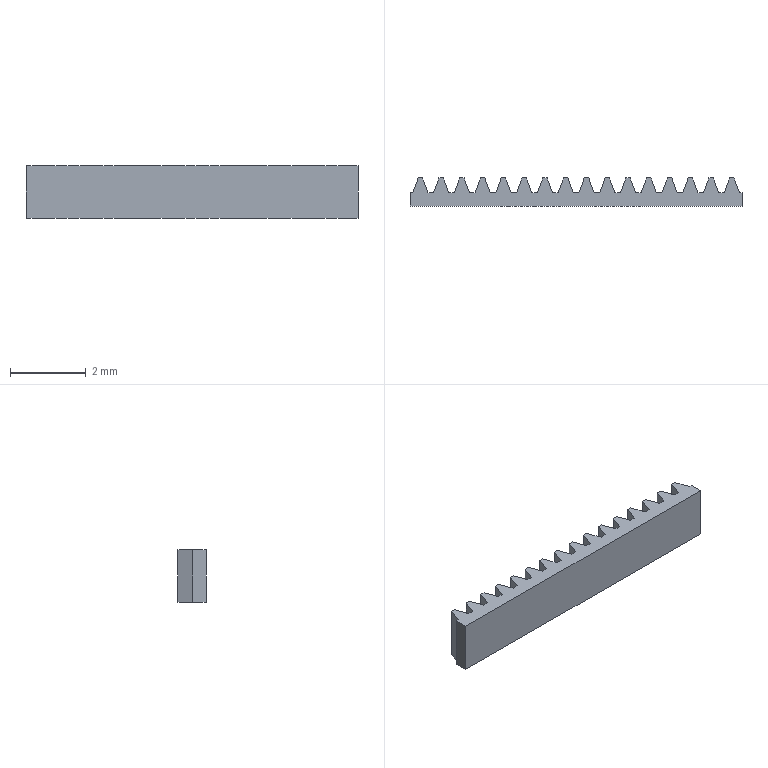Part | SolidWorks | features Extrusion 1, ICE 1, Scale 1 | 1 solid | 70 faces | box 8.791 x 0.7439 x 1.4 mm | volume 6.578 mm3 | plane 70